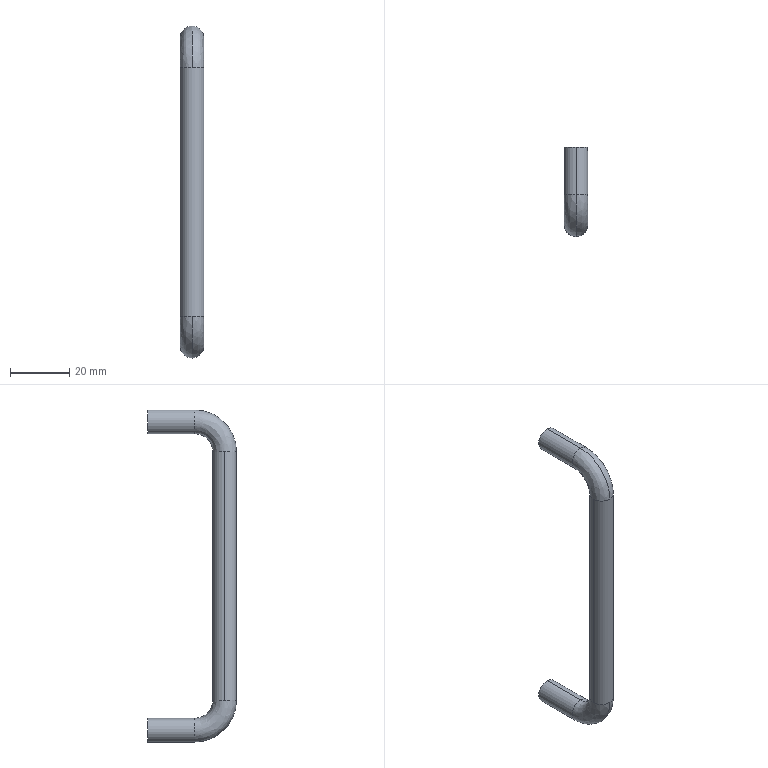Part | STEP file | Stainless steel handle | 1 solid | 20 faces | box 8 x 30 x 112 mm | volume 7163 mm3 | cylinder 10 | cone 4 | spline 4 | plane 2 | commonest cylinder face diameters 8 x6 3.3 x4